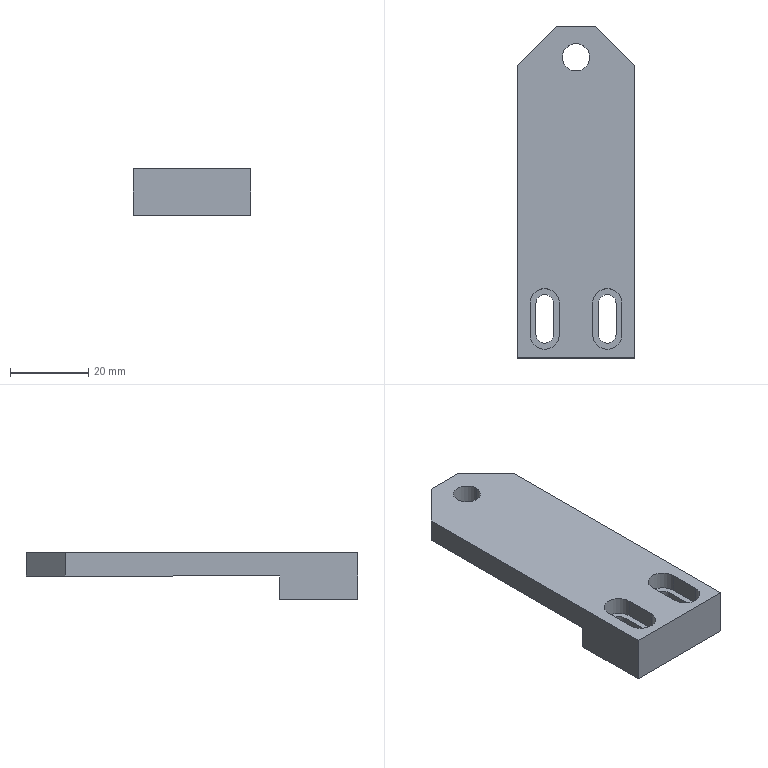Part | STEP file | BPSP-03-036Proximity Switch Mounting Plate | 1 solid | 30 faces | box 30 x 85 x 12 mm | volume 16342 mm3 | plane 20 | cylinder 10 | commonest cylinder face diameters 4.5 x4 7.5 x4 7 x2